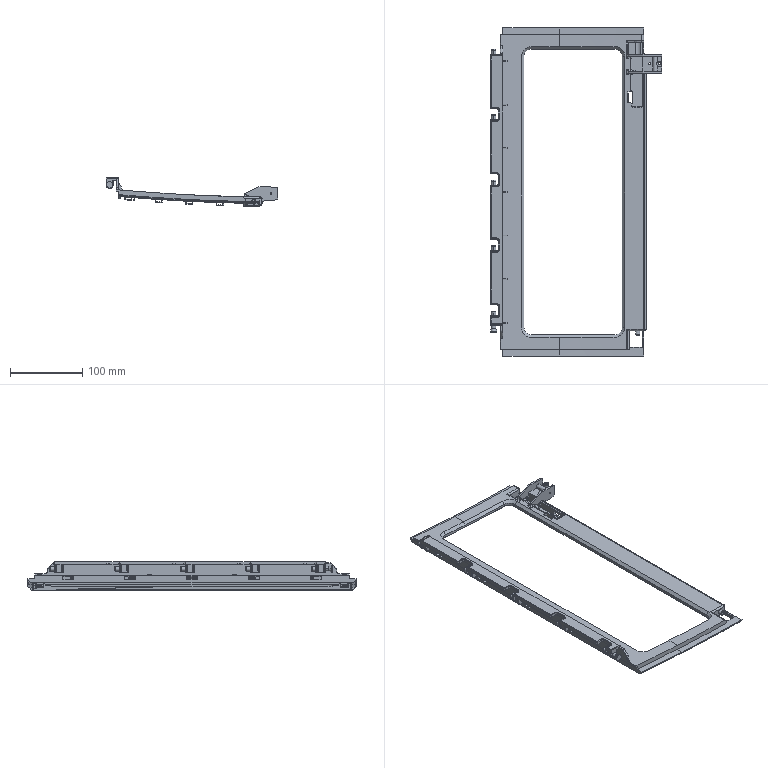Part | STEP file | solid 83 | 1 solid | 1309 faces | box 237.532 x 453.356 x 39.446 mm | volume 189015 mm3 | plane 730 | cylinder 354 | torus 110 | spline 85 | cone 28 | sphere 2 | commonest cylinder face diameters 1.005 x91 0.603 x70 6922 x45 4.02 x29 6.03 x13 4377 x13